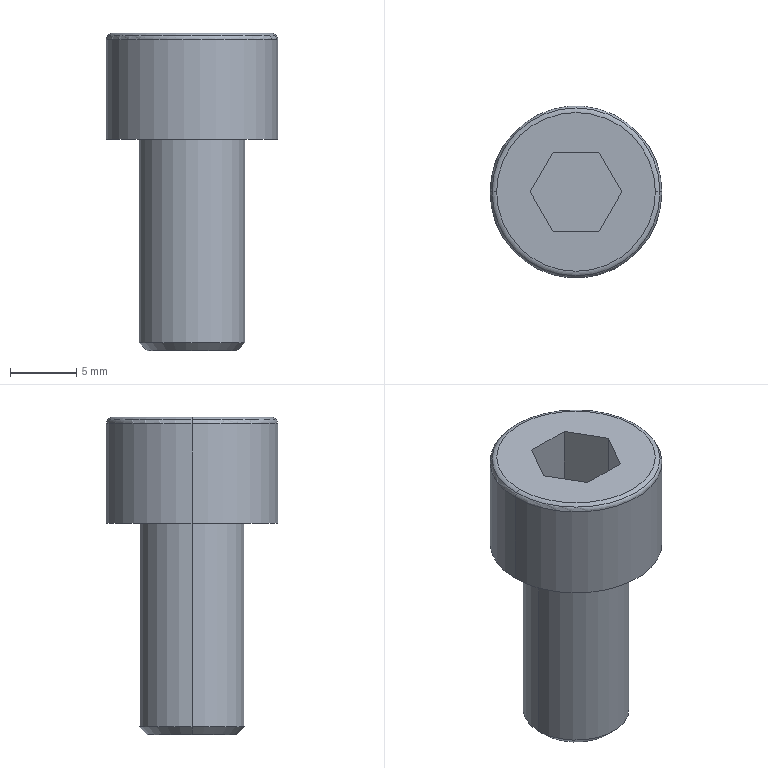Part | Creo | 1 solid | 20 faces | box 13 x 13 x 24 mm | volume 1695 mm3 | plane 10 | torus 4 | cylinder 4 | cone 2 | commonest cylinder face diameters 8 x2 13 x2
STEP:
#1=CARTESIAN_POINT('',(-119.,368.5,-22.5));
#2=VERTEX_POINT('',#1);
#3=CARTESIAN_POINT('',(-131.,368.5,-22.5));
#4=VERTEX_POINT('',#3);
#5=CARTESIAN_POINT('',(-125.,368.5,-22.5));
#6=DIRECTION('',(0.,0.,1.));
#7=DIRECTION('',(1.,0.,0.));
#8=AXIS2_PLACEMENT_3D('',#5,#6,#7);
#9=CIRCLE('',#8,6.);
#10=EDGE_CURVE('',#2,#4,#9,.T.);
#11=ORIENTED_EDGE('',*,*,#10,.F.);
#12=CARTESIAN_POINT('',(-125.,368.5,-22.5));
#13=DIRECTION('',(0.,0.,1.));
#14=DIRECTION('',(-1.,0.,0.));
#15=AXIS2_PLACEMENT_3D('',#12,#13,#14);
#16=CIRCLE('',#15,6.);
#17=EDGE_CURVE('',#4,#2,#16,.T.);
#18=ORIENTED_EDGE('',*,*,#17,.F.);
#19=EDGE_LOOP('',(#11,#18));
#20=FACE_OUTER_BOUND('',#19,.F.);
#21=CARTESIAN_POINT('',(-123.268,365.5,-22.5));
#22=VERTEX_POINT('',#21);
#23=CARTESIAN_POINT('',(-126.732,365.5,-22.5));
#24=VERTEX_POINT('',#23);
#25=CARTESIAN_POINT('',(-123.268,365.5,-22.5));
#26=DIRECTION('',(-1.,0.,0.));
#27=VECTOR('',#26,3.464);
#28=LINE('',#25,#27);
#29=EDGE_CURVE('',#22,#24,#28,.T.);
#30=ORIENTED_EDGE('',*,*,#29,.F.);
#31=CARTESIAN_POINT('',(-121.536,368.5,-22.5));
#32=VERTEX_POINT('',#31);
#33=CARTESIAN_POINT('',(-121.536,368.5,-22.5));
#34=DIRECTION('',(-0.5,-0.866,0.));
#35=VECTOR('',#34,3.464);
#36=LINE('',#33,#35);
#37=EDGE_CURVE('',#32,#22,#36,.T.);
#38=ORIENTED_EDGE('',*,*,#37,.F.);
#39=CARTESIAN_POINT('',(-123.268,371.5,-22.5));
#40=VERTEX_POINT('',#39);
#41=CARTESIAN_POINT('',(-123.268,371.5,-22.5));
#42=DIRECTION('',(0.5,-0.866,0.));
#43=VECTOR('',#42,3.464);
#44=LINE('',#41,#43);
#45=EDGE_CURVE('',#40,#32,#44,.T.);
#46=ORIENTED_EDGE('',*,*,#45,.F.);
#47=CARTESIAN_POINT('',(-126.732,371.5,-22.5));
#48=VERTEX_POINT('',#47);
#49=CARTESIAN_POINT('',(-126.732,371.5,-22.5));
#50=DIRECTION('',(1.,0.,0.));
#51=VECTOR('',#50,3.464);
#52=LINE('',#49,#51);
#53=EDGE_CURVE('',#48,#40,#52,.T.);
#54=ORIENTED_EDGE('',*,*,#53,.F.);
#55=CARTESIAN_POINT('',(-128.464,368.5,-22.5));
#56=VERTEX_POINT('',#55);
#57=CARTESIAN_POINT('',(-128.464,368.5,-22.5));
#58=DIRECTION('',(0.5,0.866,0.));
#59=VECTOR('',#58,3.464);
#60=LINE('',#57,#59);
#61=EDGE_CURVE('',#56,#48,#60,.T.);
#62=ORIENTED_EDGE('',*,*,#61,.F.);
#63=CARTESIAN_POINT('',(-126.732,365.5,-22.5));
#64=DIRECTION('',(-0.5,0.866,0.));
#65=VECTOR('',#64,3.464);
#66=LINE('',#63,#65);
#67=EDGE_CURVE('',#24,#56,#66,.T.);
#68=ORIENTED_EDGE('',*,*,#67,.F.);
#69=EDGE_LOOP('',(#30,#38,#46,#54,#62,#68));
#70=FACE_BOUND('',#69,.F.);
#71=CARTESIAN_POINT('',(-125.,368.5,-22.5));
#72=DIRECTION('',(0.,0.,1.));
#73=DIRECTION('',(1.,0.,0.));
#74=AXIS2_PLACEMENT_3D('',#71,#72,#73);
#75=PLANE('',#74);
#76=ADVANCED_FACE('',(#20,#70),#75,.T.);
#77=ORIENTED_EDGE('',*,*,#10,.T.);
#78=CARTESIAN_POINT('',(-131.354,368.5,-22.646));
#79=VERTEX_POINT('',#78);
#80=CARTESIAN_POINT('',(-131.,368.5,-23.));
#81=DIRECTION('',(0.,1.,0.));
#82=DIRECTION('',(-0.7071,0.,0.7071));
#83=AXIS2_PLACEMENT_3D('',#80,#81,#82);
#84=CIRCLE('',#83,0.5);
#85=EDGE_CURVE('',#79,#4,#84,.T.);
#86=ORIENTED_EDGE('',*,*,#85,.F.);
#87=CARTESIAN_POINT('',(-118.646,368.5,-22.646));
#88=VERTEX_POINT('',#87);
#89=CARTESIAN_POINT('',(-125.,368.5,-22.646));
#90=DIRECTION('',(0.,0.,1.));
#91=DIRECTION('',(1.,0.,0.));
#92=AXIS2_PLACEMENT_3D('',#89,#90,#91);
#93=CIRCLE('',#92,6.354);
#94=EDGE_CURVE('',#88,#79,#93,.T.);
#95=ORIENTED_EDGE('',*,*,#94,.F.);
#96=CARTESIAN_POINT('',(-119.,368.5,-23.));
#97=DIRECTION('',(0.,-1.,0.));
#98=DIRECTION('',(0.7071,0.,0.7071));
#99=AXIS2_PLACEMENT_3D('',#96,#97,#98);
#100=CIRCLE('',#99,0.5);
#101=EDGE_CURVE('',#88,#2,#100,.T.);
#102=ORIENTED_EDGE('',*,*,#101,.T.);
#103=EDGE_LOOP('',(#77,#86,#95,#102));
#104=FACE_OUTER_BOUND('',#103,.F.);
#105=CARTESIAN_POINT('',(-125.,368.5,-23.));
#106=DIRECTION('',(0.,0.,1.));
#107=DIRECTION('',(1.,0.,0.));
#108=AXIS2_PLACEMENT_3D('',#105,#106,#107);
#109=TOROIDAL_SURFACE('',#108,6.,0.5);
#110=ADVANCED_FACE('',(#104),#109,.T.);
#111=ORIENTED_EDGE('',*,*,#17,.T.);
#112=ORIENTED_EDGE('',*,*,#101,.F.);
#113=CARTESIAN_POINT('',(-125.,368.5,-22.646));
#114=DIRECTION('',(0.,0.,1.));
#115=DIRECTION('',(-1.,0.,0.));
#116=AXIS2_PLACEMENT_3D('',#113,#114,#115);
#117=CIRCLE('',#116,6.354);
#118=EDGE_CURVE('',#79,#88,#117,.T.);
#119=ORIENTED_EDGE('',*,*,#118,.F.);
#120=ORIENTED_EDGE('',*,*,#85,.T.);
#121=EDGE_LOOP('',(#111,#112,#119,#120));
#122=FACE_OUTER_BOUND('',#121,.F.);
#123=CARTESIAN_POINT('',(-125.,368.5,-23.));
#124=DIRECTION('',(0.,0.,1.));
#125=DIRECTION('',(1.,0.,0.));
#126=AXIS2_PLACEMENT_3D('',#123,#124,#125);
#127=TOROIDAL_SURFACE('',#126,6.,0.5);
#128=ADVANCED_FACE('',(#122),#127,.T.);
#129=CARTESIAN_POINT('',(-131.5,368.5,-23.));
#130=VERTEX_POINT('',#129);
#131=CARTESIAN_POINT('',(-118.5,368.5,-23.));
#132=VERTEX_POINT('',#131);
#133=CARTESIAN_POINT('',(-125.,368.5,-23.));
#134=DIRECTION('',(0.,0.,1.));
#135=DIRECTION('',(-1.,0.,0.));
#136=AXIS2_PLACEMENT_3D('',#133,#134,#135);
#137=CIRCLE('',#136,6.5);
#138=EDGE_CURVE('',#130,#132,#137,.T.);
#139=ORIENTED_EDGE('',*,*,#138,.F.);
#140=CARTESIAN_POINT('',(-131.,368.5,-23.));
#141=DIRECTION('',(0.,1.,0.));
#142=DIRECTION('',(-1.,0.,0.));
#143=AXIS2_PLACEMENT_3D('',#140,#141,#142);
#144=CIRCLE('',#143,0.5);
#145=EDGE_CURVE('',#130,#79,#144,.T.);
#146=ORIENTED_EDGE('',*,*,#145,.T.);
#147=ORIENTED_EDGE('',*,*,#118,.T.);
#148=CARTESIAN_POINT('',(-119.,368.5,-23.));
#149=DIRECTION('',(0.,-1.,0.));
#150=DIRECTION('',(1.,0.,0.));
#151=AXIS2_PLACEMENT_3D('',#148,#149,#150);
#152=CIRCLE('',#151,0.5);
#153=EDGE_CURVE('',#132,#88,#152,.T.);
#154=ORIENTED_EDGE('',*,*,#153,.F.);
#155=EDGE_LOOP('',(#139,#146,#147,#154));
#156=FACE_OUTER_BOUND('',#155,.F.);
#157=CARTESIAN_POINT('',(-125.,368.5,-23.));
#158=DIRECTION('',(0.,0.,1.));
#159=DIRECTION('',(1.,0.,0.));
#160=AXIS2_PLACEMENT_3D('',#157,#158,#159);
#161=TOROIDAL_SURFACE('',#160,6.,0.5);
#162=ADVANCED_FACE('',(#156),#161,.T.);
#163=ORIENTED_EDGE('',*,*,#138,.T.);
#164=CARTESIAN_POINT('',(-118.5,368.5,-30.5));
#165=VERTEX_POINT('',#164);
#166=CARTESIAN_POINT('',(-118.5,368.5,-30.5));
#167=DIRECTION('',(0.,0.,1.));
#168=VECTOR('',#167,7.5);
#169=LINE('',#166,#168);
#170=EDGE_CURVE('',#165,#132,#169,.T.);
#171=ORIENTED_EDGE('',*,*,#170,.F.);
#172=CARTESIAN_POINT('',(-131.5,368.5,-30.5));
#173=VERTEX_POINT('',#172);
#174=CARTESIAN_POINT('',(-125.,368.5,-30.5));
#175=DIRECTION('',(0.,0.,-1.));
#176=DIRECTION('',(1.,0.,0.));
#177=AXIS2_PLACEMENT_3D('',#174,#175,#176);
#178=CIRCLE('',#177,6.5);
#179=EDGE_CURVE('',#165,#173,#178,.T.);
#180=ORIENTED_EDGE('',*,*,#179,.T.);
#181=CARTESIAN_POINT('',(-131.5,368.5,-30.5));
#182=DIRECTION('',(0.,0.,1.));
#183=VECTOR('',#182,7.5);
#184=LINE('',#181,#183);
#185=EDGE_CURVE('',#173,#130,#184,.T.);
#186=ORIENTED_EDGE('',*,*,#185,.T.);
#187=EDGE_LOOP('',(#163,#171,#180,#186));
#188=FACE_OUTER_BOUND('',#187,.F.);
#189=CARTESIAN_POINT('',(-125.,368.5,-30.5));
#190=DIRECTION('',(0.,0.,1.));
#191=DIRECTION('',(1.,0.,0.));
#192=AXIS2_PLACEMENT_3D('',#189,#190,#191);
#193=CYLINDRICAL_SURFACE('',#192,6.5);
#194=ADVANCED_FACE('',(#188),#193,.T.);
#195=CARTESIAN_POINT('',(-125.,368.5,-23.));
#196=DIRECTION('',(0.,0.,1.));
#197=DIRECTION('',(1.,0.,0.));
#198=AXIS2_PLACEMENT_3D('',#195,#196,#197);
#199=CIRCLE('',#198,6.5);
#200=EDGE_CURVE('',#132,#130,#199,.T.);
#201=ORIENTED_EDGE('',*,*,#200,.T.);
#202=ORIENTED_EDGE('',*,*,#185,.F.);
#203=CARTESIAN_POINT('',(-125.,368.5,-30.5));
#204=DIRECTION('',(0.,0.,-1.));
#205=DIRECTION('',(-1.,0.,0.));
#206=AXIS2_PLACEMENT_3D('',#203,#204,#205);
#207=CIRCLE('',#206,6.5);
#208=EDGE_CURVE('',#173,#165,#207,.T.);
#209=ORIENTED_EDGE('',*,*,#208,.T.);
#210=ORIENTED_EDGE('',*,*,#170,.T.);
#211=EDGE_LOOP('',(#201,#202,#209,#210));
#212=FACE_OUTER_BOUND('',#211,.F.);
#213=CARTESIAN_POINT('',(-125.,368.5,-30.5));
#214=DIRECTION('',(0.,0.,1.));
#215=DIRECTION('',(1.,0.,0.));
#216=AXIS2_PLACEMENT_3D('',#213,#214,#215);
#217=CYLINDRICAL_SURFACE('',#216,6.5);
#218=ADVANCED_FACE('',(#212),#217,.T.);
#219=ORIENTED_EDGE('',*,*,#200,.F.);
#220=ORIENTED_EDGE('',*,*,#153,.T.);
#221=ORIENTED_EDGE('',*,*,#94,.T.);
#222=ORIENTED_EDGE('',*,*,#145,.F.);
#223=EDGE_LOOP('',(#219,#220,#221,#222));
#224=FACE_OUTER_BOUND('',#223,.F.);
#225=CARTESIAN_POINT('',(-125.,368.5,-23.));
#226=DIRECTION('',(0.,0.,1.));
#227=DIRECTION('',(1.,0.,0.));
#228=AXIS2_PLACEMENT_3D('',#225,#226,#227);
#229=TOROIDAL_SURFACE('',#228,6.,0.5);
#230=ADVANCED_FACE('',(#224),#229,.T.);
#231=ORIENTED_EDGE('',*,*,#179,.F.);
#232=ORIENTED_EDGE('',*,*,#208,.F.);
#233=EDGE_LOOP('',(#231,#232));
#234=FACE_OUTER_BOUND('',#233,.F.);
#235=CARTESIAN_POINT('',(-121.,368.5,-30.5));
#236=VERTEX_POINT('',#235);
#237=CARTESIAN_POINT('',(-129.,368.5,-30.5));
#238=VERTEX_POINT('',#237);
#239=CARTESIAN_POINT('',(-125.,368.5,-30.5));
#240=DIRECTION('',(0.,0.,1.));
#241=DIRECTION('',(1.,0.,0.));
#242=AXIS2_PLACEMENT_3D('',#239,#240,#241);
#243=CIRCLE('',#242,4.);
#244=EDGE_CURVE('',#236,#238,#243,.T.);
#245=ORIENTED_EDGE('',*,*,#244,.F.);
#246=CARTESIAN_POINT('',(-125.,368.5,-30.5));
#247=DIRECTION('',(0.,0.,1.));
#248=DIRECTION('',(-1.,0.,0.));
#249=AXIS2_PLACEMENT_3D('',#246,#247,#248);
#250=CIRCLE('',#249,4.);
#251=EDGE_CURVE('',#238,#236,#250,.T.);
#252=ORIENTED_EDGE('',*,*,#251,.F.);
#253=EDGE_LOOP('',(#245,#252));
#254=FACE_BOUND('',#253,.F.);
#255=CARTESIAN_POINT('',(-125.,368.5,-30.5));
#256=DIRECTION('',(0.,0.,-1.));
#257=DIRECTION('',(-1.,0.,0.));
#258=AXIS2_PLACEMENT_3D('',#255,#256,#257);
#259=PLANE('',#258);
#260=ADVANCED_FACE('',(#234,#254),#259,.T.);
#261=CARTESIAN_POINT('',(-129.,368.5,-45.9));
#262=VERTEX_POINT('',#261);
#263=CARTESIAN_POINT('',(-121.,368.5,-45.9));
#264=VERTEX_POINT('',#263);
#265=CARTESIAN_POINT('',(-125.,368.5,-45.9));
#266=DIRECTION('',(0.,0.,-1.));
#267=DIRECTION('',(-1.,0.,0.));
#268=AXIS2_PLACEMENT_3D('',#265,#266,#267);
#269=CIRCLE('',#268,4.);
#270=EDGE_CURVE('',#262,#264,#269,.T.);
#271=ORIENTED_EDGE('',*,*,#270,.T.);
#272=CARTESIAN_POINT('',(-121.,368.5,-45.9));
#273=DIRECTION('',(0.,0.,1.));
#274=VECTOR('',#273,15.4);
#275=LINE('',#272,#274);
#276=EDGE_CURVE('',#264,#236,#275,.T.);
#277=ORIENTED_EDGE('',*,*,#276,.T.);
#278=ORIENTED_EDGE('',*,*,#244,.T.);
#279=CARTESIAN_POINT('',(-129.,368.5,-45.9));
#280=DIRECTION('',(0.,0.,1.));
#281=VECTOR('',#280,15.4);
#282=LINE('',#279,#281);
#283=EDGE_CURVE('',#262,#238,#282,.T.);
#284=ORIENTED_EDGE('',*,*,#283,.F.);
#285=EDGE_LOOP('',(#271,#277,#278,#284));
#286=FACE_OUTER_BOUND('',#285,.F.);
#287=CARTESIAN_POINT('',(-125.,368.5,-46.5));
#288=DIRECTION('',(0.,0.,1.));
#289=DIRECTION('',(1.,0.,0.));
#290=AXIS2_PLACEMENT_3D('',#287,#288,#289);
#291=CYLINDRICAL_SURFACE('',#290,4.);
#292=ADVANCED_FACE('',(#286),#291,.T.);
#293=CARTESIAN_POINT('',(-128.4,368.5,-46.5));
#294=VERTEX_POINT('',#293);
#295=CARTESIAN_POINT('',(-121.6,368.5,-46.5));
#296=VERTEX_POINT('',#295);
#297=CARTESIAN_POINT('',(-125.,368.5,-46.5));
#298=DIRECTION('',(0.,0.,-1.));
#299=DIRECTION('',(-1.,0.,0.));
#300=AXIS2_PLACEMENT_3D('',#297,#298,#299);
#301=CIRCLE('',#300,3.4);
#302=EDGE_CURVE('',#294,#296,#301,.T.);
#303=ORIENTED_EDGE('',*,*,#302,.T.);
#304=CARTESIAN_POINT('',(-121.6,368.5,-46.5));
#305=DIRECTION('',(0.7071,0.,0.7071));
#306=VECTOR('',#305,0.8485);
#307=LINE('',#304,#306);
#308=EDGE_CURVE('',#296,#264,#307,.T.);
#309=ORIENTED_EDGE('',*,*,#308,.T.);
#310=ORIENTED_EDGE('',*,*,#270,.F.);
#311=CARTESIAN_POINT('',(-128.4,368.5,-46.5));
#312=DIRECTION('',(-0.7071,0.,0.7071));
#313=VECTOR('',#312,0.8485);
#314=LINE('',#311,#313);
#315=EDGE_CURVE('',#294,#262,#314,.T.);
#316=ORIENTED_EDGE('',*,*,#315,.F.);
#317=EDGE_LOOP('',(#303,#309,#310,#316));
#318=FACE_OUTER_BOUND('',#317,.F.);
#319=CARTESIAN_POINT('',(-125.,368.5,-46.2));
#320=DIRECTION('',(0.,0.,1.));
#321=DIRECTION('',(1.,0.,0.));
#322=AXIS2_PLACEMENT_3D('',#319,#320,#321);
#323=CONICAL_SURFACE('',#322,3.7,45.);
#324=ADVANCED_FACE('',(#318),#323,.T.);
#325=CARTESIAN_POINT('',(-125.,368.5,-46.5));
#326=DIRECTION('',(0.,0.,-1.));
#327=DIRECTION('',(1.,0.,0.));
#328=AXIS2_PLACEMENT_3D('',#325,#326,#327);
#329=CIRCLE('',#328,3.4);
#330=EDGE_CURVE('',#296,#294,#329,.T.);
#331=ORIENTED_EDGE('',*,*,#330,.F.);
#332=ORIENTED_EDGE('',*,*,#302,.F.);
#333=EDGE_LOOP('',(#331,#332));
#334=FACE_OUTER_BOUND('',#333,.F.);
#335=CARTESIAN_POINT('',(-125.,368.5,-46.5));
#336=DIRECTION('',(0.,0.,1.));
#337=DIRECTION('',(1.,0.,0.));
#338=AXIS2_PLACEMENT_3D('',#335,#336,#337);
#339=PLANE('',#338);
#340=ADVANCED_FACE('',(#334),#339,.F.);
#341=ORIENTED_EDGE('',*,*,#330,.T.);
#342=ORIENTED_EDGE('',*,*,#315,.T.);
#343=CARTESIAN_POINT('',(-125.,368.5,-45.9));
#344=DIRECTION('',(0.,0.,-1.));
#345=DIRECTION('',(1.,0.,0.));
#346=AXIS2_PLACEMENT_3D('',#343,#344,#345);
#347=CIRCLE('',#346,4.);
#348=EDGE_CURVE('',#264,#262,#347,.T.);
#349=ORIENTED_EDGE('',*,*,#348,.F.);
#350=ORIENTED_EDGE('',*,*,#308,.F.);
#351=EDGE_LOOP('',(#341,#342,#349,#350));
#352=FACE_OUTER_BOUND('',#351,.F.);
#353=CARTESIAN_POINT('',(-125.,368.5,-46.2));
#354=DIRECTION('',(0.,0.,1.));
#355=DIRECTION('',(1.,0.,0.));
#356=AXIS2_PLACEMENT_3D('',#353,#354,#355);
#357=CONICAL_SURFACE('',#356,3.7,45.);
#358=ADVANCED_FACE('',(#352),#357,.T.);
#359=ORIENTED_EDGE('',*,*,#348,.T.);
#360=ORIENTED_EDGE('',*,*,#283,.T.);
#361=ORIENTED_EDGE('',*,*,#251,.T.);
#362=ORIENTED_EDGE('',*,*,#276,.F.);
#363=EDGE_LOOP('',(#359,#360,#361,#362));
#364=FACE_OUTER_BOUND('',#363,.F.);
#365=CARTESIAN_POINT('',(-125.,368.5,-46.5));
#366=DIRECTION('',(0.,0.,1.));
#367=DIRECTION('',(1.,0.,0.));
#368=AXIS2_PLACEMENT_3D('',#365,#366,#367);
#369=CYLINDRICAL_SURFACE('',#368,4.);
#370=ADVANCED_FACE('',(#364),#369,.T.);
#371=ORIENTED_EDGE('',*,*,#29,.T.);
#372=CARTESIAN_POINT('',(-126.732,365.5,-27.78));
#373=VERTEX_POINT('',#372);
#374=CARTESIAN_POINT('',(-126.732,365.5,-22.5));
#375=DIRECTION('',(0.,0.,-1.));
#376=VECTOR('',#375,5.28);
#377=LINE('',#374,#376);
#378=EDGE_CURVE('',#24,#373,#377,.T.);
#379=ORIENTED_EDGE('',*,*,#378,.T.);
#380=CARTESIAN_POINT('',(-123.268,365.5,-27.78));
#381=VERTEX_POINT('',#380);
#382=CARTESIAN_POINT('',(-123.268,365.5,-27.78));
#383=DIRECTION('',(-1.,0.,0.));
#384=VECTOR('',#383,3.464);
#385=LINE('',#382,#384);
#386=EDGE_CURVE('',#381,#373,#385,.T.);
#387=ORIENTED_EDGE('',*,*,#386,.F.);
#388=CARTESIAN_POINT('',(-123.268,365.5,-22.5));
#389=DIRECTION('',(0.,0.,-1.));
#390=VECTOR('',#389,5.28);
#391=LINE('',#388,#390);
#392=EDGE_CURVE('',#22,#381,#391,.T.);
#393=ORIENTED_EDGE('',*,*,#392,.F.);
#394=EDGE_LOOP('',(#371,#379,#387,#393));
#395=FACE_OUTER_BOUND('',#394,.F.);
#396=CARTESIAN_POINT('',(-126.732,365.5,-27.78));
#397=DIRECTION('',(0.,1.,0.));
#398=DIRECTION('',(0.,0.,-1.));
#399=AXIS2_PLACEMENT_3D('',#396,#397,#398);
#400=PLANE('',#399);
#401=ADVANCED_FACE('',(#395),#400,.T.);
#402=ORIENTED_EDGE('',*,*,#67,.T.);
#403=CARTESIAN_POINT('',(-128.464,368.5,-27.78));
#404=VERTEX_POINT('',#403);
#405=CARTESIAN_POINT('',(-128.464,368.5,-22.5));
#406=DIRECTION('',(0.,0.,-1.));
#407=VECTOR('',#406,5.28);
#408=LINE('',#405,#407);
#409=EDGE_CURVE('',#56,#404,#408,.T.);
#410=ORIENTED_EDGE('',*,*,#409,.T.);
#411=CARTESIAN_POINT('',(-128.464,368.5,-27.78));
#412=DIRECTION('',(0.5,-0.866,0.));
#413=VECTOR('',#412,3.464);
#414=LINE('',#411,#413);
#415=EDGE_CURVE('',#404,#373,#414,.T.);
#416=ORIENTED_EDGE('',*,*,#415,.T.);
#417=ORIENTED_EDGE('',*,*,#378,.F.);
#418=EDGE_LOOP('',(#402,#410,#416,#417));
#419=FACE_OUTER_BOUND('',#418,.F.);
#420=CARTESIAN_POINT('',(-128.464,368.5,-27.78));
#421=DIRECTION('',(0.866,0.5,0.));
#422=DIRECTION('',(0.5,-0.866,0.));
#423=AXIS2_PLACEMENT_3D('',#420,#421,#422);
#424=PLANE('',#423);
#425=ADVANCED_FACE('',(#419),#424,.T.);
#426=ORIENTED_EDGE('',*,*,#61,.T.);
#427=CARTESIAN_POINT('',(-126.732,371.5,-27.78));
#428=VERTEX_POINT('',#427);
#429=CARTESIAN_POINT('',(-126.732,371.5,-22.5));
#430=DIRECTION('',(0.,0.,-1.));
#431=VECTOR('',#430,5.28);
#432=LINE('',#429,#431);
#433=EDGE_CURVE('',#48,#428,#432,.T.);
#434=ORIENTED_EDGE('',*,*,#433,.T.);
#435=CARTESIAN_POINT('',(-126.732,371.5,-27.78));
#436=DIRECTION('',(-0.5,-0.866,0.));
#437=VECTOR('',#436,3.464);
#438=LINE('',#435,#437);
#439=EDGE_CURVE('',#428,#404,#438,.T.);
#440=ORIENTED_EDGE('',*,*,#439,.T.);
#441=ORIENTED_EDGE('',*,*,#409,.F.);
#442=EDGE_LOOP('',(#426,#434,#440,#441));
#443=FACE_OUTER_BOUND('',#442,.F.);
#444=CARTESIAN_POINT('',(-126.732,371.5,-27.78));
#445=DIRECTION('',(0.866,-0.5,0.));
#446=DIRECTION('',(-0.5,-0.866,0.));
#447=AXIS2_PLACEMENT_3D('',#444,#445,#446);
#448=PLANE('',#447);
#449=ADVANCED_FACE('',(#443),#448,.T.);
#450=ORIENTED_EDGE('',*,*,#53,.T.);
#451=CARTESIAN_POINT('',(-123.268,371.5,-27.78));
#452=VERTEX_POINT('',#451);
#453=CARTESIAN_POINT('',(-123.268,371.5,-22.5));
#454=DIRECTION('',(0.,0.,-1.));
#455=VECTOR('',#454,5.28);
#456=LINE('',#453,#455);
#457=EDGE_CURVE('',#40,#452,#456,.T.);
#458=ORIENTED_EDGE('',*,*,#457,.T.);
#459=CARTESIAN_POINT('',(-126.732,371.5,-27.78));
#460=DIRECTION('',(1.,0.,0.));
#461=VECTOR('',#460,3.464);
#462=LINE('',#459,#461);
#463=EDGE_CURVE('',#428,#452,#462,.T.);
#464=ORIENTED_EDGE('',*,*,#463,.F.);
#465=ORIENTED_EDGE('',*,*,#433,.F.);
#466=EDGE_LOOP('',(#450,#458,#464,#465));
#467=FACE_OUTER_BOUND('',#466,.F.);
#468=CARTESIAN_POINT('',(-123.268,371.5,-27.78));
#469=DIRECTION('',(0.,-1.,0.));
#470=DIRECTION('',(0.,0.,1.));
#471=AXIS2_PLACEMENT_3D('',#468,#469,#470);
#472=PLANE('',#471);
#473=ADVANCED_FACE('',(#467),#472,.T.);
#474=ORIENTED_EDGE('',*,*,#45,.T.);
#475=CARTESIAN_POINT('',(-121.536,368.5,-27.78));
#476=VERTEX_POINT('',#475);
#477=CARTESIAN_POINT('',(-121.536,368.5,-22.5));
#478=DIRECTION('',(0.,0.,-1.));
#479=VECTOR('',#478,5.28);
#480=LINE('',#477,#479);
#481=EDGE_CURVE('',#32,#476,#480,.T.);
#482=ORIENTED_EDGE('',*,*,#481,.T.);
#483=CARTESIAN_POINT('',(-121.536,368.5,-27.78));
#484=DIRECTION('',(-0.5,0.866,0.));
#485=VECTOR('',#484,3.464);
#486=LINE('',#483,#485);
#487=EDGE_CURVE('',#476,#452,#486,.T.);
#488=ORIENTED_EDGE('',*,*,#487,.T.);
#489=ORIENTED_EDGE('',*,*,#457,.F.);
#490=EDGE_LOOP('',(#474,#482,#488,#489));
#491=FACE_OUTER_BOUND('',#490,.F.);
#492=CARTESIAN_POINT('',(-121.536,368.5,-27.78));
#493=DIRECTION('',(-0.866,-0.5,0.));
#494=DIRECTION('',(-0.5,0.866,0.));
#495=AXIS2_PLACEMENT_3D('',#492,#493,#494);
#496=PLANE('',#495);
#497=ADVANCED_FACE('',(#491),#496,.T.);
#498=ORIENTED_EDGE('',*,*,#37,.T.);
#499=ORIENTED_EDGE('',*,*,#392,.T.);
#500=CARTESIAN_POINT('',(-123.268,365.5,-27.78));
#501=DIRECTION('',(0.5,0.866,0.));
#502=VECTOR('',#501,3.464);
#503=LINE('',#500,#502);
#504=EDGE_CURVE('',#381,#476,#503,.T.);
#505=ORIENTED_EDGE('',*,*,#504,.T.);
#506=ORIENTED_EDGE('',*,*,#481,.F.);
#507=EDGE_LOOP('',(#498,#499,#505,#506));
#508=FACE_OUTER_BOUND('',#507,.F.);
#509=CARTESIAN_POINT('',(-123.268,365.5,-27.78));
#510=DIRECTION('',(-0.866,0.5,0.));
#511=DIRECTION('',(0.5,0.866,0.));
#512=AXIS2_PLACEMENT_3D('',#509,#510,#511);
#513=PLANE('',#512);
#514=ADVANCED_FACE('',(#508),#513,.T.);
#515=ORIENTED_EDGE('',*,*,#504,.F.);
#516=ORIENTED_EDGE('',*,*,#386,.T.);
#517=ORIENTED_EDGE('',*,*,#415,.F.);
#518=ORIENTED_EDGE('',*,*,#439,.F.);
#519=ORIENTED_EDGE('',*,*,#463,.T.);
#520=ORIENTED_EDGE('',*,*,#487,.F.);
#521=EDGE_LOOP('',(#515,#516,#517,#518,#519,#520));
#522=FACE_OUTER_BOUND('',#521,.F.);
#523=CARTESIAN_POINT('',(-119.804,371.5,-27.78));
#524=DIRECTION('',(0.,0.,-1.));
#525=DIRECTION('',(-1.,0.,0.));
#526=AXIS2_PLACEMENT_3D('',#523,#524,#525);
#527=PLANE('',#526);
#528=ADVANCED_FACE('',(#522),#527,.F.);
#529=CLOSED_SHELL('',(#76,#110,#128,#162,#194,#218,#230,#260,#292,#324,#340,#358,#370,#401,#425,#449,#473,#497,#514,#528));
#530=MANIFOLD_SOLID_BREP('',#529);
#531=(LENGTH_UNIT()NAMED_UNIT(*)SI_UNIT(.MILLI.,.METRE.));
#532=UNCERTAINTY_MEASURE_WITH_UNIT(LENGTH_MEASURE(0.003024),#531,'','');
#533=(NAMED_UNIT(*)PLANE_ANGLE_UNIT()SI_UNIT($,.RADIAN.));
#534=PLANE_ANGLE_MEASURE_WITH_UNIT(PLANE_ANGLE_MEASURE(0.01745),#533);
#535=(CONVERSION_BASED_UNIT('DEGREE',#534)NAMED_UNIT(*)PLANE_ANGLE_UNIT());
#536=(NAMED_UNIT(*)SI_UNIT($,.STERADIAN.)SOLID_ANGLE_UNIT());
#537=(GEOMETRIC_REPRESENTATION_CONTEXT(3)GLOBAL_UNCERTAINTY_ASSIGNED_CONTEXT((#532))GLOBAL_UNIT_ASSIGNED_CONTEXT((#531,#535,#536))REPRESENTATION_CONTEXT('',''));
#538=ADVANCED_BREP_SHAPE_REPRESENTATION('',(#530),#537);